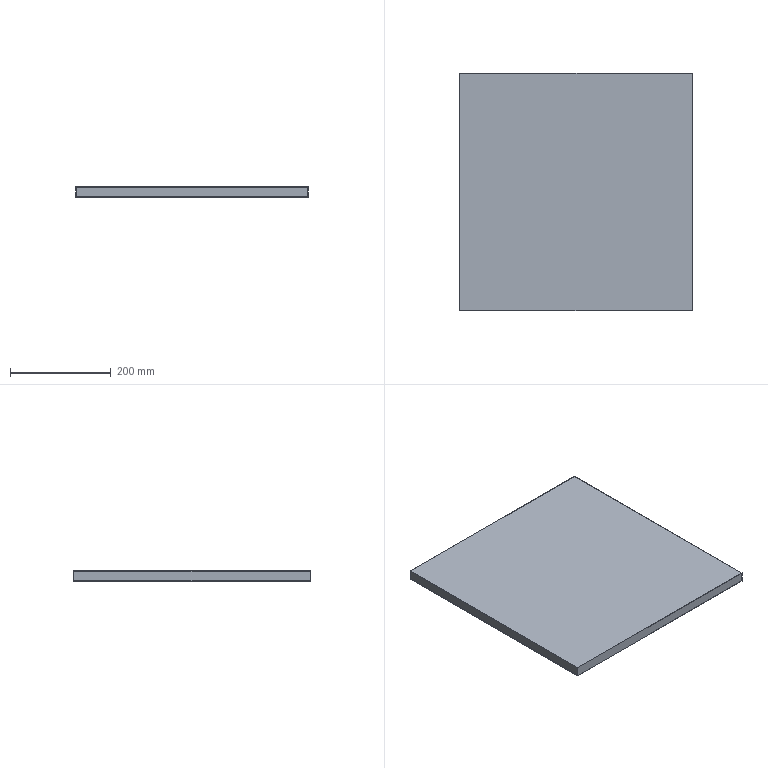Part | SolidWorks | features Cut 4, Boss 3, Extrusion 1, Fillet 1, LibraryFeature 1, MirrorPattern 1, Shell 1 | 1 solid | 16 faces | box 460 x 470 x 20 mm | volume 276608 mm3 | plane 16
STEP:
#1=CARTESIAN_POINT('',(-230.,235.,-10.));
#2=VERTEX_POINT('',#1);
#3=CARTESIAN_POINT('',(-230.,-235.,-10.));
#4=VERTEX_POINT('',#3);
#5=CARTESIAN_POINT('',(-230.,235.,-10.));
#6=DIRECTION('',(0.,-1.,0.));
#7=VECTOR('',#6,1000.);
#8=LINE('',#5,#7);
#9=EDGE_CURVE('',#2,#4,#8,.T.);
#10=ORIENTED_EDGE('',*,*,#9,.T.);
#11=CARTESIAN_POINT('',(-230.,-235.,10.));
#12=VERTEX_POINT('',#11);
#13=CARTESIAN_POINT('',(-230.,-235.,10.));
#14=DIRECTION('',(0.,0.,-1.));
#15=VECTOR('',#14,1000.);
#16=LINE('',#13,#15);
#17=EDGE_CURVE('',#12,#4,#16,.T.);
#18=ORIENTED_EDGE('',*,*,#17,.F.);
#19=CARTESIAN_POINT('',(-230.,235.,10.));
#20=VERTEX_POINT('',#19);
#21=CARTESIAN_POINT('',(-230.,235.,10.));
#22=DIRECTION('',(0.,-1.,0.));
#23=VECTOR('',#22,1000.);
#24=LINE('',#21,#23);
#25=EDGE_CURVE('',#20,#12,#24,.T.);
#26=ORIENTED_EDGE('',*,*,#25,.F.);
#27=CARTESIAN_POINT('',(-230.,235.,10.));
#28=DIRECTION('',(0.,0.,-1.));
#29=VECTOR('',#28,1000.);
#30=LINE('',#27,#29);
#31=EDGE_CURVE('',#20,#2,#30,.T.);
#32=ORIENTED_EDGE('',*,*,#31,.T.);
#33=EDGE_LOOP('',(#10,#18,#26,#32));
#34=FACE_OUTER_BOUND('',#33,.T.);
#35=CARTESIAN_POINT('',(-230.,235.,10.));
#36=DIRECTION('',(1.,0.,0.));
#37=DIRECTION('',(0.,1.,0.));
#38=AXIS2_PLACEMENT_3D('',#35,#36,#37);
#39=PLANE('',#38);
#40=ADVANCED_FACE('',(#34),#39,.F.);
#41=CARTESIAN_POINT('',(230.,-235.,-10.));
#42=VERTEX_POINT('',#41);
#43=CARTESIAN_POINT('',(-230.,-235.,-10.));
#44=DIRECTION('',(1.,0.,0.));
#45=VECTOR('',#44,1000.);
#46=LINE('',#43,#45);
#47=EDGE_CURVE('',#4,#42,#46,.T.);
#48=ORIENTED_EDGE('',*,*,#47,.T.);
#49=CARTESIAN_POINT('',(230.,-235.,10.));
#50=VERTEX_POINT('',#49);
#51=CARTESIAN_POINT('',(230.,-235.,10.));
#52=DIRECTION('',(0.,0.,-1.));
#53=VECTOR('',#52,1000.);
#54=LINE('',#51,#53);
#55=EDGE_CURVE('',#50,#42,#54,.T.);
#56=ORIENTED_EDGE('',*,*,#55,.F.);
#57=CARTESIAN_POINT('',(-230.,-235.,10.));
#58=DIRECTION('',(1.,0.,0.));
#59=VECTOR('',#58,1000.);
#60=LINE('',#57,#59);
#61=EDGE_CURVE('',#12,#50,#60,.T.);
#62=ORIENTED_EDGE('',*,*,#61,.F.);
#63=ORIENTED_EDGE('',*,*,#17,.T.);
#64=EDGE_LOOP('',(#48,#56,#62,#63));
#65=FACE_OUTER_BOUND('',#64,.T.);
#66=CARTESIAN_POINT('',(-230.,-235.,10.));
#67=DIRECTION('',(0.,1.,0.));
#68=DIRECTION('',(0.,0.,1.));
#69=AXIS2_PLACEMENT_3D('',#66,#67,#68);
#70=PLANE('',#69);
#71=ADVANCED_FACE('',(#65),#70,.F.);
#72=CARTESIAN_POINT('',(230.,235.,-10.));
#73=VERTEX_POINT('',#72);
#74=CARTESIAN_POINT('',(230.,235.,-10.));
#75=DIRECTION('',(0.,1.,0.));
#76=VECTOR('',#75,1000.);
#77=LINE('',#74,#76);
#78=EDGE_CURVE('',#42,#73,#77,.T.);
#79=ORIENTED_EDGE('',*,*,#78,.T.);
#80=CARTESIAN_POINT('',(230.,235.,10.));
#81=VERTEX_POINT('',#80);
#82=CARTESIAN_POINT('',(230.,235.,10.));
#83=DIRECTION('',(0.,0.,-1.));
#84=VECTOR('',#83,1000.);
#85=LINE('',#82,#84);
#86=EDGE_CURVE('',#81,#73,#85,.T.);
#87=ORIENTED_EDGE('',*,*,#86,.F.);
#88=CARTESIAN_POINT('',(230.,235.,10.));
#89=DIRECTION('',(0.,1.,0.));
#90=VECTOR('',#89,1000.);
#91=LINE('',#88,#90);
#92=EDGE_CURVE('',#50,#81,#91,.T.);
#93=ORIENTED_EDGE('',*,*,#92,.F.);
#94=ORIENTED_EDGE('',*,*,#55,.T.);
#95=EDGE_LOOP('',(#79,#87,#93,#94));
#96=FACE_OUTER_BOUND('',#95,.T.);
#97=CARTESIAN_POINT('',(230.,235.,10.));
#98=DIRECTION('',(-1.,0.,0.));
#99=DIRECTION('',(0.,-1.,0.));
#100=AXIS2_PLACEMENT_3D('',#97,#98,#99);
#101=PLANE('',#100);
#102=ADVANCED_FACE('',(#96),#101,.F.);
#103=CARTESIAN_POINT('',(-230.,235.,-10.));
#104=DIRECTION('',(-1.,0.,0.));
#105=VECTOR('',#104,1000.);
#106=LINE('',#103,#105);
#107=EDGE_CURVE('',#73,#2,#106,.T.);
#108=ORIENTED_EDGE('',*,*,#107,.T.);
#109=ORIENTED_EDGE('',*,*,#31,.F.);
#110=CARTESIAN_POINT('',(-230.,235.,10.));
#111=DIRECTION('',(-1.,0.,0.));
#112=VECTOR('',#111,1000.);
#113=LINE('',#110,#112);
#114=EDGE_CURVE('',#81,#20,#113,.T.);
#115=ORIENTED_EDGE('',*,*,#114,.F.);
#116=ORIENTED_EDGE('',*,*,#86,.T.);
#117=EDGE_LOOP('',(#108,#109,#115,#116));
#118=FACE_OUTER_BOUND('',#117,.T.);
#119=CARTESIAN_POINT('',(-230.,235.,10.));
#120=DIRECTION('',(0.,-1.,0.));
#121=DIRECTION('',(0.,0.,-1.));
#122=AXIS2_PLACEMENT_3D('',#119,#120,#121);
#123=PLANE('',#122);
#124=ADVANCED_FACE('',(#118),#123,.F.);
#125=ORIENTED_EDGE('',*,*,#25,.T.);
#126=ORIENTED_EDGE('',*,*,#61,.T.);
#127=ORIENTED_EDGE('',*,*,#92,.T.);
#128=ORIENTED_EDGE('',*,*,#114,.T.);
#129=EDGE_LOOP('',(#125,#126,#127,#128));
#130=FACE_OUTER_BOUND('',#129,.T.);
#131=CARTESIAN_POINT('',(-230.,-235.,10.));
#132=DIRECTION('',(0.,0.,1.));
#133=DIRECTION('',(1.,0.,0.));
#134=AXIS2_PLACEMENT_3D('',#131,#132,#133);
#135=PLANE('',#134);
#136=ADVANCED_FACE('',(#130),#135,.T.);
#137=CARTESIAN_POINT('',(-215.,-220.,-10.));
#138=VERTEX_POINT('',#137);
#139=CARTESIAN_POINT('',(-215.,220.,-10.));
#140=VERTEX_POINT('',#139);
#141=CARTESIAN_POINT('',(-215.,-220.,-10.));
#142=DIRECTION('',(0.,1.,0.));
#143=VECTOR('',#142,1000.);
#144=LINE('',#141,#143);
#145=EDGE_CURVE('',#138,#140,#144,.T.);
#146=ORIENTED_EDGE('',*,*,#145,.F.);
#147=CARTESIAN_POINT('',(215.,-220.,-10.));
#148=VERTEX_POINT('',#147);
#149=CARTESIAN_POINT('',(215.,-220.,-10.));
#150=DIRECTION('',(-1.,0.,0.));
#151=VECTOR('',#150,1000.);
#152=LINE('',#149,#151);
#153=EDGE_CURVE('',#148,#138,#152,.T.);
#154=ORIENTED_EDGE('',*,*,#153,.F.);
#155=CARTESIAN_POINT('',(215.,220.,-10.));
#156=VERTEX_POINT('',#155);
#157=CARTESIAN_POINT('',(215.,220.,-10.));
#158=DIRECTION('',(0.,-1.,0.));
#159=VECTOR('',#158,1000.);
#160=LINE('',#157,#159);
#161=EDGE_CURVE('',#156,#148,#160,.T.);
#162=ORIENTED_EDGE('',*,*,#161,.F.);
#163=CARTESIAN_POINT('',(-215.,220.,-10.));
#164=DIRECTION('',(1.,0.,0.));
#165=VECTOR('',#164,1000.);
#166=LINE('',#163,#165);
#167=EDGE_CURVE('',#140,#156,#166,.T.);
#168=ORIENTED_EDGE('',*,*,#167,.F.);
#169=EDGE_LOOP('',(#146,#154,#162,#168));
#170=FACE_BOUND('',#169,.T.);
#171=ORIENTED_EDGE('',*,*,#9,.F.);
#172=ORIENTED_EDGE('',*,*,#107,.F.);
#173=ORIENTED_EDGE('',*,*,#78,.F.);
#174=ORIENTED_EDGE('',*,*,#47,.F.);
#175=EDGE_LOOP('',(#171,#172,#173,#174));
#176=FACE_OUTER_BOUND('',#175,.T.);
#177=CARTESIAN_POINT('',(-230.,-235.,-10.));
#178=DIRECTION('',(0.,0.,1.));
#179=DIRECTION('',(1.,0.,0.));
#180=AXIS2_PLACEMENT_3D('',#177,#178,#179);
#181=PLANE('',#180);
#182=ADVANCED_FACE('',(#170,#176),#181,.F.);
#183=ORIENTED_EDGE('',*,*,#153,.T.);
#184=CARTESIAN_POINT('',(-215.,-220.,-9.));
#185=VERTEX_POINT('',#184);
#186=CARTESIAN_POINT('',(-215.,-220.,-9.));
#187=DIRECTION('',(0.,0.,-1.));
#188=VECTOR('',#187,1000.);
#189=LINE('',#186,#188);
#190=EDGE_CURVE('',#185,#138,#189,.T.);
#191=ORIENTED_EDGE('',*,*,#190,.F.);
#192=CARTESIAN_POINT('',(215.,-220.,-9.));
#193=VERTEX_POINT('',#192);
#194=CARTESIAN_POINT('',(215.,-220.,-9.));
#195=DIRECTION('',(-1.,0.,0.));
#196=VECTOR('',#195,1000.);
#197=LINE('',#194,#196);
#198=EDGE_CURVE('',#193,#185,#197,.T.);
#199=ORIENTED_EDGE('',*,*,#198,.F.);
#200=CARTESIAN_POINT('',(215.,-220.,-9.));
#201=DIRECTION('',(0.,0.,-1.));
#202=VECTOR('',#201,1000.);
#203=LINE('',#200,#202);
#204=EDGE_CURVE('',#193,#148,#203,.T.);
#205=ORIENTED_EDGE('',*,*,#204,.T.);
#206=EDGE_LOOP('',(#183,#191,#199,#205));
#207=FACE_OUTER_BOUND('',#206,.T.);
#208=CARTESIAN_POINT('',(215.,-220.,-9.));
#209=DIRECTION('',(0.,-1.,0.));
#210=DIRECTION('',(0.,0.,-1.));
#211=AXIS2_PLACEMENT_3D('',#208,#209,#210);
#212=PLANE('',#211);
#213=ADVANCED_FACE('',(#207),#212,.F.);
#214=ORIENTED_EDGE('',*,*,#161,.T.);
#215=ORIENTED_EDGE('',*,*,#204,.F.);
#216=CARTESIAN_POINT('',(215.,220.,-9.));
#217=VERTEX_POINT('',#216);
#218=CARTESIAN_POINT('',(215.,220.,-9.));
#219=DIRECTION('',(0.,-1.,0.));
#220=VECTOR('',#219,1000.);
#221=LINE('',#218,#220);
#222=EDGE_CURVE('',#217,#193,#221,.T.);
#223=ORIENTED_EDGE('',*,*,#222,.F.);
#224=CARTESIAN_POINT('',(215.,220.,-9.));
#225=DIRECTION('',(0.,0.,-1.));
#226=VECTOR('',#225,1000.);
#227=LINE('',#224,#226);
#228=EDGE_CURVE('',#217,#156,#227,.T.);
#229=ORIENTED_EDGE('',*,*,#228,.T.);
#230=EDGE_LOOP('',(#214,#215,#223,#229));
#231=FACE_OUTER_BOUND('',#230,.T.);
#232=CARTESIAN_POINT('',(215.,220.,-9.));
#233=DIRECTION('',(1.,0.,0.));
#234=DIRECTION('',(0.,1.,0.));
#235=AXIS2_PLACEMENT_3D('',#232,#233,#234);
#236=PLANE('',#235);
#237=ADVANCED_FACE('',(#231),#236,.F.);
#238=ORIENTED_EDGE('',*,*,#167,.T.);
#239=ORIENTED_EDGE('',*,*,#228,.F.);
#240=CARTESIAN_POINT('',(-215.,220.,-9.));
#241=VERTEX_POINT('',#240);
#242=CARTESIAN_POINT('',(-215.,220.,-9.));
#243=DIRECTION('',(1.,0.,0.));
#244=VECTOR('',#243,1000.);
#245=LINE('',#242,#244);
#246=EDGE_CURVE('',#241,#217,#245,.T.);
#247=ORIENTED_EDGE('',*,*,#246,.F.);
#248=CARTESIAN_POINT('',(-215.,220.,-9.));
#249=DIRECTION('',(0.,0.,-1.));
#250=VECTOR('',#249,1000.);
#251=LINE('',#248,#250);
#252=EDGE_CURVE('',#241,#140,#251,.T.);
#253=ORIENTED_EDGE('',*,*,#252,.T.);
#254=EDGE_LOOP('',(#238,#239,#247,#253));
#255=FACE_OUTER_BOUND('',#254,.T.);
#256=CARTESIAN_POINT('',(-215.,220.,-9.));
#257=DIRECTION('',(0.,1.,0.));
#258=DIRECTION('',(0.,0.,1.));
#259=AXIS2_PLACEMENT_3D('',#256,#257,#258);
#260=PLANE('',#259);
#261=ADVANCED_FACE('',(#255),#260,.F.);
#262=ORIENTED_EDGE('',*,*,#145,.T.);
#263=ORIENTED_EDGE('',*,*,#252,.F.);
#264=CARTESIAN_POINT('',(-215.,-220.,-9.));
#265=DIRECTION('',(0.,1.,0.));
#266=VECTOR('',#265,1000.);
#267=LINE('',#264,#266);
#268=EDGE_CURVE('',#185,#241,#267,.T.);
#269=ORIENTED_EDGE('',*,*,#268,.F.);
#270=ORIENTED_EDGE('',*,*,#190,.T.);
#271=EDGE_LOOP('',(#262,#263,#269,#270));
#272=FACE_OUTER_BOUND('',#271,.T.);
#273=CARTESIAN_POINT('',(-215.,-220.,-9.));
#274=DIRECTION('',(-1.,0.,0.));
#275=DIRECTION('',(0.,-1.,0.));
#276=AXIS2_PLACEMENT_3D('',#273,#274,#275);
#277=PLANE('',#276);
#278=ADVANCED_FACE('',(#272),#277,.F.);
#279=CARTESIAN_POINT('',(-229.,234.,-9.));
#280=VERTEX_POINT('',#279);
#281=CARTESIAN_POINT('',(-229.,-234.,-9.));
#282=VERTEX_POINT('',#281);
#283=CARTESIAN_POINT('',(-229.,235.,-9.));
#284=DIRECTION('',(0.,-1.,0.));
#285=VECTOR('',#284,1000.);
#286=LINE('',#283,#285);
#287=EDGE_CURVE('',#280,#282,#286,.T.);
#288=ORIENTED_EDGE('',*,*,#287,.T.);
#289=CARTESIAN_POINT('',(229.,-234.,-9.));
#290=VERTEX_POINT('',#289);
#291=CARTESIAN_POINT('',(-230.,-234.,-9.));
#292=DIRECTION('',(1.,0.,0.));
#293=VECTOR('',#292,1000.);
#294=LINE('',#291,#293);
#295=EDGE_CURVE('',#282,#290,#294,.T.);
#296=ORIENTED_EDGE('',*,*,#295,.T.);
#297=CARTESIAN_POINT('',(229.,234.,-9.));
#298=VERTEX_POINT('',#297);
#299=CARTESIAN_POINT('',(229.,235.,-9.));
#300=DIRECTION('',(0.,1.,0.));
#301=VECTOR('',#300,1000.);
#302=LINE('',#299,#301);
#303=EDGE_CURVE('',#290,#298,#302,.T.);
#304=ORIENTED_EDGE('',*,*,#303,.T.);
#305=CARTESIAN_POINT('',(-230.,234.,-9.));
#306=DIRECTION('',(-1.,0.,0.));
#307=VECTOR('',#306,1000.);
#308=LINE('',#305,#307);
#309=EDGE_CURVE('',#298,#280,#308,.T.);
#310=ORIENTED_EDGE('',*,*,#309,.T.);
#311=EDGE_LOOP('',(#288,#296,#304,#310));
#312=FACE_OUTER_BOUND('',#311,.T.);
#313=ORIENTED_EDGE('',*,*,#198,.T.);
#314=ORIENTED_EDGE('',*,*,#268,.T.);
#315=ORIENTED_EDGE('',*,*,#246,.T.);
#316=ORIENTED_EDGE('',*,*,#222,.T.);
#317=EDGE_LOOP('',(#313,#314,#315,#316));
#318=FACE_BOUND('',#317,.T.);
#319=CARTESIAN_POINT('',(-230.,-235.,-9.));
#320=DIRECTION('',(0.,0.,1.));
#321=DIRECTION('',(1.,0.,0.));
#322=AXIS2_PLACEMENT_3D('',#319,#320,#321);
#323=PLANE('',#322);
#324=ADVANCED_FACE('',(#312,#318),#323,.T.);
#325=ORIENTED_EDGE('',*,*,#287,.F.);
#326=CARTESIAN_POINT('',(-229.,234.,9.));
#327=VERTEX_POINT('',#326);
#328=CARTESIAN_POINT('',(-229.,234.,10.));
#329=DIRECTION('',(0.,0.,-1.));
#330=VECTOR('',#329,1000.);
#331=LINE('',#328,#330);
#332=EDGE_CURVE('',#327,#280,#331,.T.);
#333=ORIENTED_EDGE('',*,*,#332,.F.);
#334=CARTESIAN_POINT('',(-229.,-234.,9.));
#335=VERTEX_POINT('',#334);
#336=CARTESIAN_POINT('',(-229.,235.,9.));
#337=DIRECTION('',(0.,-1.,0.));
#338=VECTOR('',#337,1000.);
#339=LINE('',#336,#338);
#340=EDGE_CURVE('',#327,#335,#339,.T.);
#341=ORIENTED_EDGE('',*,*,#340,.T.);
#342=CARTESIAN_POINT('',(-229.,-234.,10.));
#343=DIRECTION('',(0.,0.,-1.));
#344=VECTOR('',#343,1000.);
#345=LINE('',#342,#344);
#346=EDGE_CURVE('',#335,#282,#345,.T.);
#347=ORIENTED_EDGE('',*,*,#346,.T.);
#348=EDGE_LOOP('',(#325,#333,#341,#347));
#349=FACE_OUTER_BOUND('',#348,.T.);
#350=CARTESIAN_POINT('',(-229.,235.,10.));
#351=DIRECTION('',(1.,0.,0.));
#352=DIRECTION('',(0.,1.,0.));
#353=AXIS2_PLACEMENT_3D('',#350,#351,#352);
#354=PLANE('',#353);
#355=ADVANCED_FACE('',(#349),#354,.T.);
#356=ORIENTED_EDGE('',*,*,#295,.F.);
#357=ORIENTED_EDGE('',*,*,#346,.F.);
#358=CARTESIAN_POINT('',(229.,-234.,9.));
#359=VERTEX_POINT('',#358);
#360=CARTESIAN_POINT('',(-230.,-234.,9.));
#361=DIRECTION('',(1.,0.,0.));
#362=VECTOR('',#361,1000.);
#363=LINE('',#360,#362);
#364=EDGE_CURVE('',#335,#359,#363,.T.);
#365=ORIENTED_EDGE('',*,*,#364,.T.);
#366=CARTESIAN_POINT('',(229.,-234.,10.));
#367=DIRECTION('',(0.,0.,-1.));
#368=VECTOR('',#367,1000.);
#369=LINE('',#366,#368);
#370=EDGE_CURVE('',#359,#290,#369,.T.);
#371=ORIENTED_EDGE('',*,*,#370,.T.);
#372=EDGE_LOOP('',(#356,#357,#365,#371));
#373=FACE_OUTER_BOUND('',#372,.T.);
#374=CARTESIAN_POINT('',(-230.,-234.,10.));
#375=DIRECTION('',(0.,1.,0.));
#376=DIRECTION('',(0.,0.,1.));
#377=AXIS2_PLACEMENT_3D('',#374,#375,#376);
#378=PLANE('',#377);
#379=ADVANCED_FACE('',(#373),#378,.T.);
#380=ORIENTED_EDGE('',*,*,#303,.F.);
#381=ORIENTED_EDGE('',*,*,#370,.F.);
#382=CARTESIAN_POINT('',(229.,234.,9.));
#383=VERTEX_POINT('',#382);
#384=CARTESIAN_POINT('',(229.,235.,9.));
#385=DIRECTION('',(0.,1.,0.));
#386=VECTOR('',#385,1000.);
#387=LINE('',#384,#386);
#388=EDGE_CURVE('',#359,#383,#387,.T.);
#389=ORIENTED_EDGE('',*,*,#388,.T.);
#390=CARTESIAN_POINT('',(229.,234.,10.));
#391=DIRECTION('',(0.,0.,-1.));
#392=VECTOR('',#391,1000.);
#393=LINE('',#390,#392);
#394=EDGE_CURVE('',#383,#298,#393,.T.);
#395=ORIENTED_EDGE('',*,*,#394,.T.);
#396=EDGE_LOOP('',(#380,#381,#389,#395));
#397=FACE_OUTER_BOUND('',#396,.T.);
#398=CARTESIAN_POINT('',(229.,235.,10.));
#399=DIRECTION('',(-1.,0.,0.));
#400=DIRECTION('',(0.,-1.,0.));
#401=AXIS2_PLACEMENT_3D('',#398,#399,#400);
#402=PLANE('',#401);
#403=ADVANCED_FACE('',(#397),#402,.T.);
#404=ORIENTED_EDGE('',*,*,#309,.F.);
#405=ORIENTED_EDGE('',*,*,#394,.F.);
#406=CARTESIAN_POINT('',(-230.,234.,9.));
#407=DIRECTION('',(-1.,0.,0.));
#408=VECTOR('',#407,1000.);
#409=LINE('',#406,#408);
#410=EDGE_CURVE('',#383,#327,#409,.T.);
#411=ORIENTED_EDGE('',*,*,#410,.T.);
#412=ORIENTED_EDGE('',*,*,#332,.T.);
#413=EDGE_LOOP('',(#404,#405,#411,#412));
#414=FACE_OUTER_BOUND('',#413,.T.);
#415=CARTESIAN_POINT('',(-230.,234.,10.));
#416=DIRECTION('',(0.,-1.,0.));
#417=DIRECTION('',(0.,0.,-1.));
#418=AXIS2_PLACEMENT_3D('',#415,#416,#417);
#419=PLANE('',#418);
#420=ADVANCED_FACE('',(#414),#419,.T.);
#421=ORIENTED_EDGE('',*,*,#340,.F.);
#422=ORIENTED_EDGE('',*,*,#410,.F.);
#423=ORIENTED_EDGE('',*,*,#388,.F.);
#424=ORIENTED_EDGE('',*,*,#364,.F.);
#425=EDGE_LOOP('',(#421,#422,#423,#424));
#426=FACE_OUTER_BOUND('',#425,.T.);
#427=CARTESIAN_POINT('',(-230.,-235.,9.));
#428=DIRECTION('',(0.,0.,1.));
#429=DIRECTION('',(1.,0.,0.));
#430=AXIS2_PLACEMENT_3D('',#427,#428,#429);
#431=PLANE('',#430);
#432=ADVANCED_FACE('',(#426),#431,.F.);
#433=CLOSED_SHELL('',(#40,#71,#102,#124,#136,#182,#213,#237,#261,#278,#324,#355,#379,#403,#420,#432));
#434=MANIFOLD_SOLID_BREP('',#433);
#435=CARTESIAN_POINT('',(0.,0.,0.));
#436=DIRECTION('',(0.,0.,1.));
#437=DIRECTION('',(1.,0.,0.));
#438=AXIS2_PLACEMENT_3D('',#435,#436,#437);
#439=(LENGTH_UNIT()NAMED_UNIT(*)SI_UNIT(.MILLI.,.METRE.));
#440=UNCERTAINTY_MEASURE_WITH_UNIT(LENGTH_MEASURE(0.00001),#439,'','');
#441=(NAMED_UNIT(*)PLANE_ANGLE_UNIT()SI_UNIT($,.RADIAN.));
#442=(NAMED_UNIT(*)SI_UNIT($,.STERADIAN.)SOLID_ANGLE_UNIT());
#443=(GEOMETRIC_REPRESENTATION_CONTEXT(3)GLOBAL_UNCERTAINTY_ASSIGNED_CONTEXT((#440))GLOBAL_UNIT_ASSIGNED_CONTEXT((#439,#441,#442))REPRESENTATION_CONTEXT('',''));
#444=ADVANCED_BREP_SHAPE_REPRESENTATION('',(#434,#438),#443);